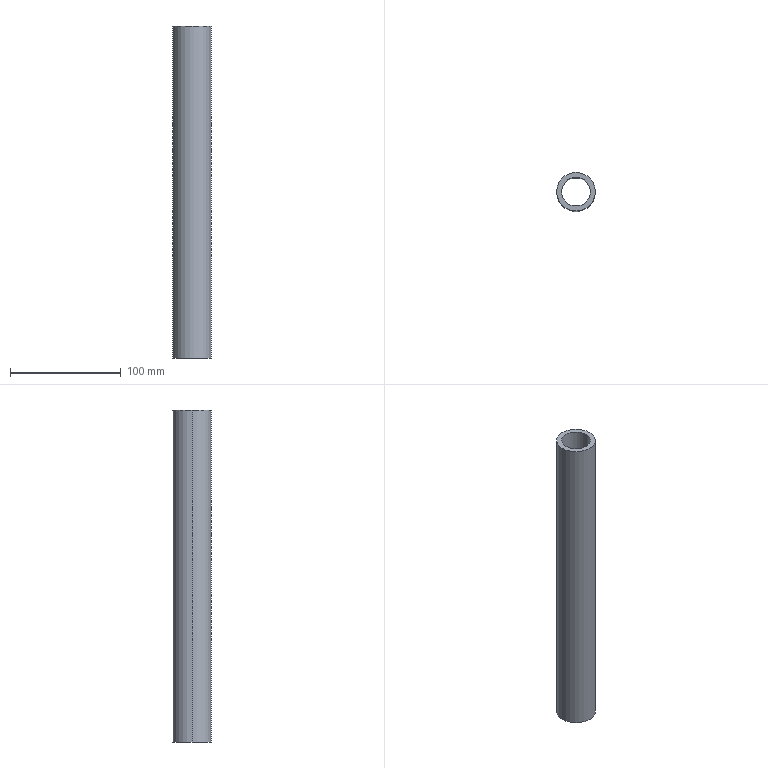Part | NX | features BREP 1 | 1 solid | 6 faces | box 35 x 35 x 300 mm | volume 129355 mm3 | cylinder 4 | plane 2 | commonest cylinder face diameters 26 x2 35 x2
STEP:
#1=CARTESIAN_POINT('',(-13.,0.,300.));
#2=VERTEX_POINT('',#1);
#3=CARTESIAN_POINT('',(13.,0.,300.));
#4=VERTEX_POINT('',#3);
#5=CARTESIAN_POINT('',(0.,0.,300.));
#6=DIRECTION('',(0.,0.,1.));
#7=DIRECTION('',(1.,0.,0.));
#8=AXIS2_PLACEMENT_3D('',#5,#6,#7);
#9=CIRCLE('',#8,13.);
#10=EDGE_CURVE('',#2,#4,#9,.T.);
#11=ORIENTED_EDGE('',*,*,#10,.T.);
#12=CARTESIAN_POINT('',(13.,0.,0.));
#13=VERTEX_POINT('',#12);
#14=CARTESIAN_POINT('',(13.,0.,300.));
#15=DIRECTION('',(0.,0.,-1.));
#16=VECTOR('',#15,1000.);
#17=LINE('',#14,#16);
#18=EDGE_CURVE('',#13,#4,#17,.F.);
#19=ORIENTED_EDGE('',*,*,#18,.F.);
#20=CARTESIAN_POINT('',(-13.,0.,0.));
#21=VERTEX_POINT('',#20);
#22=CARTESIAN_POINT('',(0.,0.,0.));
#23=DIRECTION('',(0.,0.,1.));
#24=DIRECTION('',(1.,0.,0.));
#25=AXIS2_PLACEMENT_3D('',#22,#23,#24);
#26=CIRCLE('',#25,13.);
#27=EDGE_CURVE('',#21,#13,#26,.T.);
#28=ORIENTED_EDGE('',*,*,#27,.F.);
#29=CARTESIAN_POINT('',(-13.,0.,300.));
#30=DIRECTION('',(0.,0.,-1.));
#31=VECTOR('',#30,1000.);
#32=LINE('',#29,#31);
#33=EDGE_CURVE('',#21,#2,#32,.F.);
#34=ORIENTED_EDGE('',*,*,#33,.T.);
#35=EDGE_LOOP('',(#11,#19,#28,#34));
#36=FACE_BOUND('',#35,.T.);
#37=CARTESIAN_POINT('',(0.,0.,300.));
#38=DIRECTION('',(0.,0.,-1.));
#39=DIRECTION('',(1.,0.,0.));
#40=AXIS2_PLACEMENT_3D('',#37,#38,#39);
#41=CYLINDRICAL_SURFACE('',#40,13.);
#42=ADVANCED_FACE('',(#36),#41,.F.);
#43=CARTESIAN_POINT('',(17.5,0.,300.));
#44=VERTEX_POINT('',#43);
#45=CARTESIAN_POINT('',(-17.5,0.,300.));
#46=VERTEX_POINT('',#45);
#47=CARTESIAN_POINT('',(0.,0.,300.));
#48=DIRECTION('',(0.,0.,1.));
#49=DIRECTION('',(1.,0.,0.));
#50=AXIS2_PLACEMENT_3D('',#47,#48,#49);
#51=CIRCLE('',#50,17.5);
#52=EDGE_CURVE('',#44,#46,#51,.T.);
#53=ORIENTED_EDGE('',*,*,#52,.F.);
#54=CARTESIAN_POINT('',(17.5,0.,0.));
#55=VERTEX_POINT('',#54);
#56=CARTESIAN_POINT('',(17.5,0.,300.));
#57=DIRECTION('',(0.,0.,-1.));
#58=VECTOR('',#57,1000.);
#59=LINE('',#56,#58);
#60=EDGE_CURVE('',#55,#44,#59,.F.);
#61=ORIENTED_EDGE('',*,*,#60,.F.);
#62=CARTESIAN_POINT('',(-17.5,0.,0.));
#63=VERTEX_POINT('',#62);
#64=CARTESIAN_POINT('',(0.,0.,0.));
#65=DIRECTION('',(0.,0.,1.));
#66=DIRECTION('',(1.,0.,0.));
#67=AXIS2_PLACEMENT_3D('',#64,#65,#66);
#68=CIRCLE('',#67,17.5);
#69=EDGE_CURVE('',#55,#63,#68,.T.);
#70=ORIENTED_EDGE('',*,*,#69,.T.);
#71=CARTESIAN_POINT('',(-17.5,0.,300.));
#72=DIRECTION('',(0.,0.,-1.));
#73=VECTOR('',#72,1000.);
#74=LINE('',#71,#73);
#75=EDGE_CURVE('',#63,#46,#74,.F.);
#76=ORIENTED_EDGE('',*,*,#75,.T.);
#77=EDGE_LOOP('',(#53,#61,#70,#76));
#78=FACE_BOUND('',#77,.T.);
#79=CARTESIAN_POINT('',(0.,0.,300.));
#80=DIRECTION('',(0.,0.,-1.));
#81=DIRECTION('',(1.,0.,0.));
#82=AXIS2_PLACEMENT_3D('',#79,#80,#81);
#83=CYLINDRICAL_SURFACE('',#82,17.5);
#84=ADVANCED_FACE('',(#78),#83,.T.);
#85=CARTESIAN_POINT('',(0.,0.,300.));
#86=DIRECTION('',(0.,0.,1.));
#87=DIRECTION('',(1.,0.,0.));
#88=AXIS2_PLACEMENT_3D('',#85,#86,#87);
#89=CIRCLE('',#88,17.5);
#90=EDGE_CURVE('',#46,#44,#89,.T.);
#91=ORIENTED_EDGE('',*,*,#90,.T.);
#92=ORIENTED_EDGE('',*,*,#52,.T.);
#93=EDGE_LOOP('',(#91,#92));
#94=FACE_BOUND('',#93,.T.);
#95=ORIENTED_EDGE('',*,*,#10,.F.);
#96=CARTESIAN_POINT('',(0.,0.,300.));
#97=DIRECTION('',(0.,0.,1.));
#98=DIRECTION('',(1.,0.,0.));
#99=AXIS2_PLACEMENT_3D('',#96,#97,#98);
#100=CIRCLE('',#99,13.);
#101=EDGE_CURVE('',#4,#2,#100,.T.);
#102=ORIENTED_EDGE('',*,*,#101,.F.);
#103=EDGE_LOOP('',(#95,#102));
#104=FACE_BOUND('',#103,.T.);
#105=CARTESIAN_POINT('',(0.,0.,300.));
#106=DIRECTION('',(0.,0.,1.));
#107=DIRECTION('',(-1.,0.,0.));
#108=AXIS2_PLACEMENT_3D('',#105,#106,#107);
#109=PLANE('',#108);
#110=ADVANCED_FACE('',(#94,#104),#109,.T.);
#111=CARTESIAN_POINT('',(0.,0.,0.));
#112=DIRECTION('',(0.,0.,1.));
#113=DIRECTION('',(1.,0.,0.));
#114=AXIS2_PLACEMENT_3D('',#111,#112,#113);
#115=CIRCLE('',#114,17.5);
#116=EDGE_CURVE('',#63,#55,#115,.T.);
#117=ORIENTED_EDGE('',*,*,#116,.F.);
#118=ORIENTED_EDGE('',*,*,#69,.F.);
#119=EDGE_LOOP('',(#117,#118));
#120=FACE_BOUND('',#119,.T.);
#121=ORIENTED_EDGE('',*,*,#27,.T.);
#122=CARTESIAN_POINT('',(0.,0.,0.));
#123=DIRECTION('',(0.,0.,1.));
#124=DIRECTION('',(1.,0.,0.));
#125=AXIS2_PLACEMENT_3D('',#122,#123,#124);
#126=CIRCLE('',#125,13.);
#127=EDGE_CURVE('',#13,#21,#126,.T.);
#128=ORIENTED_EDGE('',*,*,#127,.T.);
#129=EDGE_LOOP('',(#121,#128));
#130=FACE_BOUND('',#129,.T.);
#131=CARTESIAN_POINT('',(0.,0.,0.));
#132=DIRECTION('',(0.,0.,1.));
#133=DIRECTION('',(-1.,0.,0.));
#134=AXIS2_PLACEMENT_3D('',#131,#132,#133);
#135=PLANE('',#134);
#136=ADVANCED_FACE('',(#120,#130),#135,.F.);
#137=ORIENTED_EDGE('',*,*,#60,.T.);
#138=ORIENTED_EDGE('',*,*,#90,.F.);
#139=ORIENTED_EDGE('',*,*,#75,.F.);
#140=ORIENTED_EDGE('',*,*,#116,.T.);
#141=EDGE_LOOP('',(#137,#138,#139,#140));
#142=FACE_BOUND('',#141,.T.);
#143=CARTESIAN_POINT('',(0.,0.,300.));
#144=DIRECTION('',(0.,0.,-1.));
#145=DIRECTION('',(1.,0.,0.));
#146=AXIS2_PLACEMENT_3D('',#143,#144,#145);
#147=CYLINDRICAL_SURFACE('',#146,17.5);
#148=ADVANCED_FACE('',(#142),#147,.T.);
#149=ORIENTED_EDGE('',*,*,#18,.T.);
#150=ORIENTED_EDGE('',*,*,#101,.T.);
#151=ORIENTED_EDGE('',*,*,#33,.F.);
#152=ORIENTED_EDGE('',*,*,#127,.F.);
#153=EDGE_LOOP('',(#149,#150,#151,#152));
#154=FACE_BOUND('',#153,.T.);
#155=CARTESIAN_POINT('',(0.,0.,300.));
#156=DIRECTION('',(0.,0.,-1.));
#157=DIRECTION('',(1.,0.,0.));
#158=AXIS2_PLACEMENT_3D('',#155,#156,#157);
#159=CYLINDRICAL_SURFACE('',#158,13.);
#160=ADVANCED_FACE('',(#154),#159,.F.);
#161=CLOSED_SHELL('',(#42,#84,#110,#136,#148,#160));
#162=MANIFOLD_SOLID_BREP('',#161);
#163=(LENGTH_UNIT()NAMED_UNIT(*)SI_UNIT(.MILLI.,.METRE.));
#164=UNCERTAINTY_MEASURE_WITH_UNIT(LENGTH_MEASURE(0.00001),#163,'','');
#165=(NAMED_UNIT(*)PLANE_ANGLE_UNIT()SI_UNIT($,.RADIAN.));
#166=(NAMED_UNIT(*)SI_UNIT($,.STERADIAN.)SOLID_ANGLE_UNIT());
#167=(GEOMETRIC_REPRESENTATION_CONTEXT(3)GLOBAL_UNCERTAINTY_ASSIGNED_CONTEXT((#164))GLOBAL_UNIT_ASSIGNED_CONTEXT((#163,#165,#166))REPRESENTATION_CONTEXT('',''));
#168=ADVANCED_BREP_SHAPE_REPRESENTATION('',(#162),#167);